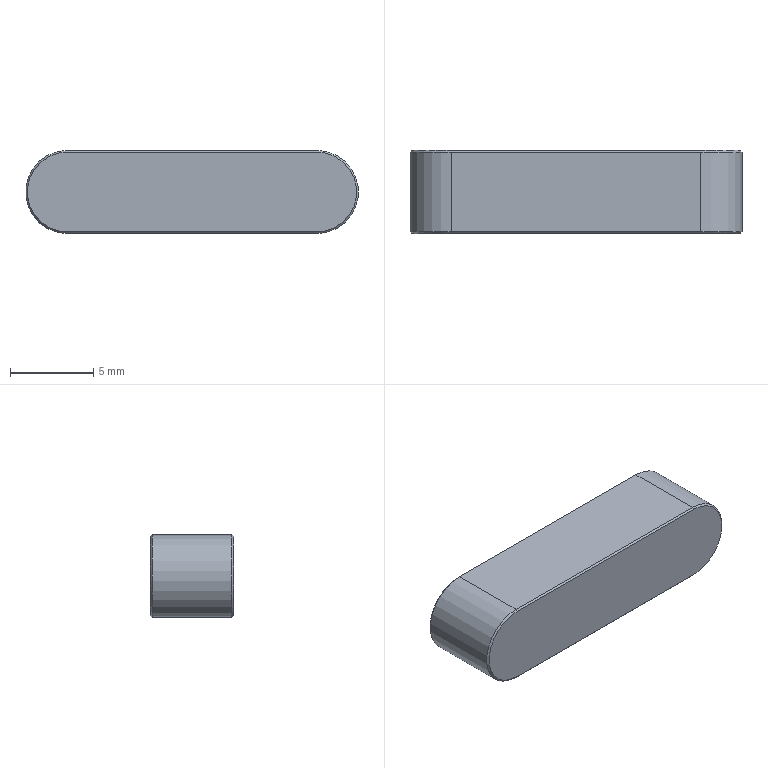Part | STEP file | Plain key (type B) 5x5x20 | 1 solid | 14 faces | box 20 x 5 x 5 mm | volume 472.72 mm3 | plane 8 | cone 4 | cylinder 2 | commonest cylinder face diameters 5 x2
STEP:
#1=CARTESIAN_POINT('',(0.,0.,0.));
#2=DIRECTION('',(0.,0.,1.));
#3=DIRECTION('',(1.,0.,0.));
#4=AXIS2_PLACEMENT_3D('',#1,#2,#3);
#5=CARTESIAN_POINT('',(-7.5,2.4,-2.5));
#6=VERTEX_POINT('',#5);
#7=CARTESIAN_POINT('',(-7.5,-2.4,-2.5));
#8=VERTEX_POINT('',#7);
#9=CARTESIAN_POINT('',(-7.5,2.5,-2.5));
#10=DIRECTION('',(0.,-1.,0.));
#11=VECTOR('',#10,1.);
#12=LINE('',#9,#11);
#13=CARTESIAN_POINT('',(-7.5,2.5,0.));
#14=DIRECTION('',(0.,-1.,0.));
#15=DIRECTION('',(0.,0.,-1.));
#16=AXIS2_PLACEMENT_3D('',#13,#14,#15);
#17=CYLINDRICAL_SURFACE('',#16,2.5);
#18=CARTESIAN_POINT('',(6.283,0.));
#19=DIRECTION('',(0.,1.));
#20=VECTOR('',#19,1.);
#21=LINE('',#18,#20);
#22=(GEOMETRIC_REPRESENTATION_CONTEXT(2)PARAMETRIC_REPRESENTATION_CONTEXT()REPRESENTATION_CONTEXT('',''));
#23=DEFINITIONAL_REPRESENTATION('',(#21),#22);
#24=PCURVE('',#17,#23);
#25=CARTESIAN_POINT('',(-7.5,2.5,-2.5));
#26=DIRECTION('',(0.,0.,1.));
#27=DIRECTION('',(1.,0.,0.));
#28=AXIS2_PLACEMENT_3D('',#25,#26,#27);
#29=PLANE('',#28);
#30=CARTESIAN_POINT('',(0.,0.));
#31=DIRECTION('',(0.,-1.));
#32=VECTOR('',#31,1.);
#33=LINE('',#30,#32);
#34=(GEOMETRIC_REPRESENTATION_CONTEXT(2)PARAMETRIC_REPRESENTATION_CONTEXT()REPRESENTATION_CONTEXT('',''));
#35=DEFINITIONAL_REPRESENTATION('',(#33),#34);
#36=PCURVE('',#29,#35);
#37=SURFACE_CURVE('',#12,(#24,#36),.PCURVE_S1.);
#38=EDGE_CURVE('',#6,#8,#37,.T.);
#39=ORIENTED_EDGE('',*,*,#38,.T.);
#40=CARTESIAN_POINT('',(-7.5,-2.4,2.5));
#41=VERTEX_POINT('',#40);
#42=CARTESIAN_POINT('',(-7.5,-2.4,0.));
#43=DIRECTION('',(0.,1.,0.));
#44=DIRECTION('',(0.,0.,1.));
#45=AXIS2_PLACEMENT_3D('',#42,#43,#44);
#46=CIRCLE('',#45,2.5);
#47=CARTESIAN_POINT('',(9.425,4.9));
#48=DIRECTION('',(-1.,0.));
#49=VECTOR('',#48,1.);
#50=LINE('',#47,#49);
#51=(GEOMETRIC_REPRESENTATION_CONTEXT(2)PARAMETRIC_REPRESENTATION_CONTEXT()REPRESENTATION_CONTEXT('',''));
#52=DEFINITIONAL_REPRESENTATION('',(#50),#51);
#53=PCURVE('',#17,#52);
#54=CARTESIAN_POINT('',(-7.5,-2.4,0.));
#55=DIRECTION('',(0.,1.,0.));
#56=DIRECTION('',(0.,0.,1.));
#57=AXIS2_PLACEMENT_3D('',#54,#55,#56);
#58=CONICAL_SURFACE('',#57,2.5,0.7854);
#59=CARTESIAN_POINT('',(0.,0.));
#60=DIRECTION('',(1.,0.));
#61=VECTOR('',#60,1.);
#62=LINE('',#59,#61);
#63=(GEOMETRIC_REPRESENTATION_CONTEXT(2)PARAMETRIC_REPRESENTATION_CONTEXT()REPRESENTATION_CONTEXT('',''));
#64=DEFINITIONAL_REPRESENTATION('',(#62),#63);
#65=PCURVE('',#58,#64);
#66=SURFACE_CURVE('',#46,(#53,#65),.PCURVE_S1.);
#67=EDGE_CURVE('',#8,#41,#66,.T.);
#68=ORIENTED_EDGE('',*,*,#67,.T.);
#69=CARTESIAN_POINT('',(-7.5,2.4,2.5));
#70=VERTEX_POINT('',#69);
#71=CARTESIAN_POINT('',(-7.5,2.5,2.5));
#72=DIRECTION('',(0.,-1.,0.));
#73=VECTOR('',#72,1.);
#74=LINE('',#71,#73);
#75=CARTESIAN_POINT('',(3.142,0.));
#76=DIRECTION('',(0.,1.));
#77=VECTOR('',#76,1.);
#78=LINE('',#75,#77);
#79=(GEOMETRIC_REPRESENTATION_CONTEXT(2)PARAMETRIC_REPRESENTATION_CONTEXT()REPRESENTATION_CONTEXT('',''));
#80=DEFINITIONAL_REPRESENTATION('',(#78),#79);
#81=PCURVE('',#17,#80);
#82=CARTESIAN_POINT('',(-7.5,2.5,2.5));
#83=DIRECTION('',(0.,0.,-1.));
#84=DIRECTION('',(-1.,0.,0.));
#85=AXIS2_PLACEMENT_3D('',#82,#83,#84);
#86=PLANE('',#85);
#87=CARTESIAN_POINT('',(0.,0.));
#88=DIRECTION('',(0.,-1.));
#89=VECTOR('',#88,1.);
#90=LINE('',#87,#89);
#91=(GEOMETRIC_REPRESENTATION_CONTEXT(2)PARAMETRIC_REPRESENTATION_CONTEXT()REPRESENTATION_CONTEXT('',''));
#92=DEFINITIONAL_REPRESENTATION('',(#90),#91);
#93=PCURVE('',#86,#92);
#94=SURFACE_CURVE('',#74,(#81,#93),.PCURVE_S1.);
#95=EDGE_CURVE('',#70,#41,#94,.T.);
#96=ORIENTED_EDGE('',*,*,#95,.F.);
#97=CARTESIAN_POINT('',(-7.5,2.4,0.));
#98=DIRECTION('',(0.,-1.,0.));
#99=DIRECTION('',(0.,0.,1.));
#100=AXIS2_PLACEMENT_3D('',#97,#98,#99);
#101=CIRCLE('',#100,2.5);
#102=CARTESIAN_POINT('',(3.142,0.1));
#103=DIRECTION('',(1.,0.));
#104=VECTOR('',#103,1.);
#105=LINE('',#102,#104);
#106=(GEOMETRIC_REPRESENTATION_CONTEXT(2)PARAMETRIC_REPRESENTATION_CONTEXT()REPRESENTATION_CONTEXT('',''));
#107=DEFINITIONAL_REPRESENTATION('',(#105),#106);
#108=PCURVE('',#17,#107);
#109=CARTESIAN_POINT('',(-7.5,2.5,0.));
#110=DIRECTION('',(0.,-1.,0.));
#111=DIRECTION('',(0.,0.,-1.));
#112=AXIS2_PLACEMENT_3D('',#109,#110,#111);
#113=CONICAL_SURFACE('',#112,2.4,0.7854);
#114=CARTESIAN_POINT('',(3.142,0.1));
#115=DIRECTION('',(1.,0.));
#116=VECTOR('',#115,1.);
#117=LINE('',#114,#116);
#118=(GEOMETRIC_REPRESENTATION_CONTEXT(2)PARAMETRIC_REPRESENTATION_CONTEXT()REPRESENTATION_CONTEXT('',''));
#119=DEFINITIONAL_REPRESENTATION('',(#117),#118);
#120=PCURVE('',#113,#119);
#121=SURFACE_CURVE('',#101,(#108,#120),.PCURVE_S1.);
#122=EDGE_CURVE('',#70,#6,#121,.T.);
#123=ORIENTED_EDGE('',*,*,#122,.T.);
#124=EDGE_LOOP('',(#39,#68,#96,#123));
#125=FACE_BOUND('',#124,.T.);
#126=ADVANCED_FACE('',(#125),#17,.T.);
#127=ORIENTED_EDGE('',*,*,#95,.T.);
#128=CARTESIAN_POINT('',(7.5,-2.4,2.5));
#129=VERTEX_POINT('',#128);
#130=CARTESIAN_POINT('',(-7.5,-2.4,2.5));
#131=DIRECTION('',(1.,0.,0.));
#132=VECTOR('',#131,1.);
#133=LINE('',#130,#132);
#134=CARTESIAN_POINT('',(0.,-4.9));
#135=DIRECTION('',(-1.,0.));
#136=VECTOR('',#135,1.);
#137=LINE('',#134,#136);
#138=(GEOMETRIC_REPRESENTATION_CONTEXT(2)PARAMETRIC_REPRESENTATION_CONTEXT()REPRESENTATION_CONTEXT('',''));
#139=DEFINITIONAL_REPRESENTATION('',(#137),#138);
#140=PCURVE('',#86,#139);
#141=CARTESIAN_POINT('',(-7.5,-2.4,2.5));
#142=DIRECTION('',(0.,0.7071,-0.7071));
#143=DIRECTION('',(1.,0.,0.));
#144=AXIS2_PLACEMENT_3D('',#141,#142,#143);
#145=PLANE('',#144);
#146=CARTESIAN_POINT('',(0.,0.));
#147=DIRECTION('',(1.,0.));
#148=VECTOR('',#147,1.);
#149=LINE('',#146,#148);
#150=(GEOMETRIC_REPRESENTATION_CONTEXT(2)PARAMETRIC_REPRESENTATION_CONTEXT()REPRESENTATION_CONTEXT('',''));
#151=DEFINITIONAL_REPRESENTATION('',(#149),#150);
#152=PCURVE('',#145,#151);
#153=SURFACE_CURVE('',#133,(#140,#152),.PCURVE_S1.);
#154=EDGE_CURVE('',#41,#129,#153,.T.);
#155=ORIENTED_EDGE('',*,*,#154,.T.);
#156=CARTESIAN_POINT('',(7.5,2.4,2.5));
#157=VERTEX_POINT('',#156);
#158=CARTESIAN_POINT('',(7.5,2.5,2.5));
#159=DIRECTION('',(0.,-1.,0.));
#160=VECTOR('',#159,1.);
#161=LINE('',#158,#160);
#162=CARTESIAN_POINT('',(-15.,0.));
#163=DIRECTION('',(0.,-1.));
#164=VECTOR('',#163,1.);
#165=LINE('',#162,#164);
#166=(GEOMETRIC_REPRESENTATION_CONTEXT(2)PARAMETRIC_REPRESENTATION_CONTEXT()REPRESENTATION_CONTEXT('',''));
#167=DEFINITIONAL_REPRESENTATION('',(#165),#166);
#168=PCURVE('',#86,#167);
#169=CARTESIAN_POINT('',(7.5,2.5,0.));
#170=DIRECTION('',(0.,-1.,0.));
#171=DIRECTION('',(0.,0.,-1.));
#172=AXIS2_PLACEMENT_3D('',#169,#170,#171);
#173=CYLINDRICAL_SURFACE('',#172,2.5);
#174=CARTESIAN_POINT('',(3.142,0.));
#175=DIRECTION('',(0.,1.));
#176=VECTOR('',#175,1.);
#177=LINE('',#174,#176);
#178=(GEOMETRIC_REPRESENTATION_CONTEXT(2)PARAMETRIC_REPRESENTATION_CONTEXT()REPRESENTATION_CONTEXT('',''));
#179=DEFINITIONAL_REPRESENTATION('',(#177),#178);
#180=PCURVE('',#173,#179);
#181=SURFACE_CURVE('',#161,(#168,#180),.PCURVE_S1.);
#182=EDGE_CURVE('',#157,#129,#181,.T.);
#183=ORIENTED_EDGE('',*,*,#182,.F.);
#184=CARTESIAN_POINT('',(-7.5,2.4,2.5));
#185=DIRECTION('',(-1.,0.,0.));
#186=VECTOR('',#185,1.);
#187=LINE('',#184,#186);
#188=CARTESIAN_POINT('',(0.,-0.1));
#189=DIRECTION('',(1.,0.));
#190=VECTOR('',#189,1.);
#191=LINE('',#188,#190);
#192=(GEOMETRIC_REPRESENTATION_CONTEXT(2)PARAMETRIC_REPRESENTATION_CONTEXT()REPRESENTATION_CONTEXT('',''));
#193=DEFINITIONAL_REPRESENTATION('',(#191),#192);
#194=PCURVE('',#86,#193);
#195=CARTESIAN_POINT('',(-7.5,2.5,2.4));
#196=DIRECTION('',(0.,0.7071,0.7071));
#197=DIRECTION('',(-1.,0.,0.));
#198=AXIS2_PLACEMENT_3D('',#195,#196,#197);
#199=PLANE('',#198);
#200=CARTESIAN_POINT('',(0.,0.1414));
#201=DIRECTION('',(1.,0.));
#202=VECTOR('',#201,1.);
#203=LINE('',#200,#202);
#204=(GEOMETRIC_REPRESENTATION_CONTEXT(2)PARAMETRIC_REPRESENTATION_CONTEXT()REPRESENTATION_CONTEXT('',''));
#205=DEFINITIONAL_REPRESENTATION('',(#203),#204);
#206=PCURVE('',#199,#205);
#207=SURFACE_CURVE('',#187,(#194,#206),.PCURVE_S1.);
#208=EDGE_CURVE('',#157,#70,#207,.T.);
#209=ORIENTED_EDGE('',*,*,#208,.T.);
#210=EDGE_LOOP('',(#127,#155,#183,#209));
#211=FACE_BOUND('',#210,.T.);
#212=ADVANCED_FACE('',(#211),#86,.F.);
#213=ORIENTED_EDGE('',*,*,#182,.T.);
#214=CARTESIAN_POINT('',(7.5,-2.4,-2.5));
#215=VERTEX_POINT('',#214);
#216=CARTESIAN_POINT('',(7.5,-2.4,0.));
#217=DIRECTION('',(0.,1.,0.));
#218=DIRECTION('',(0.,0.,1.));
#219=AXIS2_PLACEMENT_3D('',#216,#217,#218);
#220=CIRCLE('',#219,2.5);
#221=CARTESIAN_POINT('',(3.142,4.9));
#222=DIRECTION('',(-1.,0.));
#223=VECTOR('',#222,1.);
#224=LINE('',#221,#223);
#225=(GEOMETRIC_REPRESENTATION_CONTEXT(2)PARAMETRIC_REPRESENTATION_CONTEXT()REPRESENTATION_CONTEXT('',''));
#226=DEFINITIONAL_REPRESENTATION('',(#224),#225);
#227=PCURVE('',#173,#226);
#228=CARTESIAN_POINT('',(7.5,-2.4,0.));
#229=DIRECTION('',(0.,1.,0.));
#230=DIRECTION('',(0.,0.,1.));
#231=AXIS2_PLACEMENT_3D('',#228,#229,#230);
#232=CONICAL_SURFACE('',#231,2.5,0.7854);
#233=CARTESIAN_POINT('',(0.,0.));
#234=DIRECTION('',(1.,0.));
#235=VECTOR('',#234,1.);
#236=LINE('',#233,#235);
#237=(GEOMETRIC_REPRESENTATION_CONTEXT(2)PARAMETRIC_REPRESENTATION_CONTEXT()REPRESENTATION_CONTEXT('',''));
#238=DEFINITIONAL_REPRESENTATION('',(#236),#237);
#239=PCURVE('',#232,#238);
#240=SURFACE_CURVE('',#220,(#227,#239),.PCURVE_S1.);
#241=EDGE_CURVE('',#129,#215,#240,.T.);
#242=ORIENTED_EDGE('',*,*,#241,.T.);
#243=CARTESIAN_POINT('',(7.5,2.4,-2.5));
#244=VERTEX_POINT('',#243);
#245=CARTESIAN_POINT('',(7.5,2.5,-2.5));
#246=DIRECTION('',(0.,-1.,0.));
#247=VECTOR('',#246,1.);
#248=LINE('',#245,#247);
#249=CARTESIAN_POINT('',(0.,0.));
#250=DIRECTION('',(0.,1.));
#251=VECTOR('',#250,1.);
#252=LINE('',#249,#251);
#253=(GEOMETRIC_REPRESENTATION_CONTEXT(2)PARAMETRIC_REPRESENTATION_CONTEXT()REPRESENTATION_CONTEXT('',''));
#254=DEFINITIONAL_REPRESENTATION('',(#252),#253);
#255=PCURVE('',#173,#254);
#256=CARTESIAN_POINT('',(15.,0.));
#257=DIRECTION('',(0.,-1.));
#258=VECTOR('',#257,1.);
#259=LINE('',#256,#258);
#260=(GEOMETRIC_REPRESENTATION_CONTEXT(2)PARAMETRIC_REPRESENTATION_CONTEXT()REPRESENTATION_CONTEXT('',''));
#261=DEFINITIONAL_REPRESENTATION('',(#259),#260);
#262=PCURVE('',#29,#261);
#263=SURFACE_CURVE('',#248,(#255,#262),.PCURVE_S1.);
#264=EDGE_CURVE('',#244,#215,#263,.T.);
#265=ORIENTED_EDGE('',*,*,#264,.F.);
#266=CARTESIAN_POINT('',(7.5,2.4,0.));
#267=DIRECTION('',(0.,-1.,0.));
#268=DIRECTION('',(0.,0.,1.));
#269=AXIS2_PLACEMENT_3D('',#266,#267,#268);
#270=CIRCLE('',#269,2.5);
#271=CARTESIAN_POINT('',(-3.142,0.1));
#272=DIRECTION('',(1.,0.));
#273=VECTOR('',#272,1.);
#274=LINE('',#271,#273);
#275=(GEOMETRIC_REPRESENTATION_CONTEXT(2)PARAMETRIC_REPRESENTATION_CONTEXT()REPRESENTATION_CONTEXT('',''));
#276=DEFINITIONAL_REPRESENTATION('',(#274),#275);
#277=PCURVE('',#173,#276);
#278=CARTESIAN_POINT('',(7.5,2.5,0.));
#279=DIRECTION('',(0.,-1.,0.));
#280=DIRECTION('',(0.,0.,-1.));
#281=AXIS2_PLACEMENT_3D('',#278,#279,#280);
#282=CONICAL_SURFACE('',#281,2.4,0.7854);
#283=CARTESIAN_POINT('',(-3.142,0.1));
#284=DIRECTION('',(1.,0.));
#285=VECTOR('',#284,1.);
#286=LINE('',#283,#285);
#287=(GEOMETRIC_REPRESENTATION_CONTEXT(2)PARAMETRIC_REPRESENTATION_CONTEXT()REPRESENTATION_CONTEXT('',''));
#288=DEFINITIONAL_REPRESENTATION('',(#286),#287);
#289=PCURVE('',#282,#288);
#290=SURFACE_CURVE('',#270,(#277,#289),.PCURVE_S1.);
#291=EDGE_CURVE('',#244,#157,#290,.T.);
#292=ORIENTED_EDGE('',*,*,#291,.T.);
#293=EDGE_LOOP('',(#213,#242,#265,#292));
#294=FACE_BOUND('',#293,.T.);
#295=ADVANCED_FACE('',(#294),#173,.T.);
#296=ORIENTED_EDGE('',*,*,#264,.T.);
#297=CARTESIAN_POINT('',(-7.5,-2.4,-2.5));
#298=DIRECTION('',(-1.,0.,0.));
#299=VECTOR('',#298,1.);
#300=LINE('',#297,#299);
#301=CARTESIAN_POINT('',(0.,-4.9));
#302=DIRECTION('',(-1.,0.));
#303=VECTOR('',#302,1.);
#304=LINE('',#301,#303);
#305=(GEOMETRIC_REPRESENTATION_CONTEXT(2)PARAMETRIC_REPRESENTATION_CONTEXT()REPRESENTATION_CONTEXT('',''));
#306=DEFINITIONAL_REPRESENTATION('',(#304),#305);
#307=PCURVE('',#29,#306);
#308=CARTESIAN_POINT('',(-7.5,-2.4,-2.5));
#309=DIRECTION('',(0.,0.7071,0.7071));
#310=DIRECTION('',(-1.,0.,0.));
#311=AXIS2_PLACEMENT_3D('',#308,#309,#310);
#312=PLANE('',#311);
#313=CARTESIAN_POINT('',(0.,0.));
#314=DIRECTION('',(1.,0.));
#315=VECTOR('',#314,1.);
#316=LINE('',#313,#315);
#317=(GEOMETRIC_REPRESENTATION_CONTEXT(2)PARAMETRIC_REPRESENTATION_CONTEXT()REPRESENTATION_CONTEXT('',''));
#318=DEFINITIONAL_REPRESENTATION('',(#316),#317);
#319=PCURVE('',#312,#318);
#320=SURFACE_CURVE('',#300,(#307,#319),.PCURVE_S1.);
#321=EDGE_CURVE('',#215,#8,#320,.T.);
#322=ORIENTED_EDGE('',*,*,#321,.T.);
#323=ORIENTED_EDGE('',*,*,#38,.F.);
#324=CARTESIAN_POINT('',(7.5,2.4,-2.5));
#325=DIRECTION('',(1.,0.,0.));
#326=VECTOR('',#325,1.);
#327=LINE('',#324,#326);
#328=CARTESIAN_POINT('',(15.,-0.1));
#329=DIRECTION('',(1.,0.));
#330=VECTOR('',#329,1.);
#331=LINE('',#328,#330);
#332=(GEOMETRIC_REPRESENTATION_CONTEXT(2)PARAMETRIC_REPRESENTATION_CONTEXT()REPRESENTATION_CONTEXT('',''));
#333=DEFINITIONAL_REPRESENTATION('',(#331),#332);
#334=PCURVE('',#29,#333);
#335=CARTESIAN_POINT('',(-7.5,2.5,-2.4));
#336=DIRECTION('',(0.,0.7071,-0.7071));
#337=DIRECTION('',(1.,0.,0.));
#338=AXIS2_PLACEMENT_3D('',#335,#336,#337);
#339=PLANE('',#338);
#340=CARTESIAN_POINT('',(15.,0.1414));
#341=DIRECTION('',(1.,0.));
#342=VECTOR('',#341,1.);
#343=LINE('',#340,#342);
#344=(GEOMETRIC_REPRESENTATION_CONTEXT(2)PARAMETRIC_REPRESENTATION_CONTEXT()REPRESENTATION_CONTEXT('',''));
#345=DEFINITIONAL_REPRESENTATION('',(#343),#344);
#346=PCURVE('',#339,#345);
#347=SURFACE_CURVE('',#327,(#334,#346),.PCURVE_S1.);
#348=EDGE_CURVE('',#6,#244,#347,.T.);
#349=ORIENTED_EDGE('',*,*,#348,.T.);
#350=EDGE_LOOP('',(#296,#322,#323,#349));
#351=FACE_BOUND('',#350,.T.);
#352=ADVANCED_FACE('',(#351),#29,.F.);
#353=CARTESIAN_POINT('',(-7.5,2.5,-2.4));
#354=VERTEX_POINT('',#353);
#355=CARTESIAN_POINT('',(-7.5,2.5,2.4));
#356=VERTEX_POINT('',#355);
#357=CARTESIAN_POINT('',(-7.5,2.5,0.));
#358=DIRECTION('',(0.,1.,0.));
#359=DIRECTION('',(0.,0.,1.));
#360=AXIS2_PLACEMENT_3D('',#357,#358,#359);
#361=CIRCLE('',#360,2.4);
#362=CARTESIAN_POINT('',(-7.5,2.5,0.));
#363=DIRECTION('',(0.,1.,0.));
#364=DIRECTION('',(0.,0.,1.));
#365=AXIS2_PLACEMENT_3D('',#362,#363,#364);
#366=PLANE('',#365);
#367=CARTESIAN_POINT('',(0.,0.));
#368=DIRECTION('',(1.,0.));
#369=AXIS2_PLACEMENT_2D('',#367,#368);
#370=CIRCLE('',#369,2.4);
#371=(GEOMETRIC_REPRESENTATION_CONTEXT(2)PARAMETRIC_REPRESENTATION_CONTEXT()REPRESENTATION_CONTEXT('',''));
#372=DEFINITIONAL_REPRESENTATION('',(#370),#371);
#373=PCURVE('',#366,#372);
#374=CARTESIAN_POINT('',(9.425,0.));
#375=DIRECTION('',(-1.,0.));
#376=VECTOR('',#375,1.);
#377=LINE('',#374,#376);
#378=(GEOMETRIC_REPRESENTATION_CONTEXT(2)PARAMETRIC_REPRESENTATION_CONTEXT()REPRESENTATION_CONTEXT('',''));
#379=DEFINITIONAL_REPRESENTATION('',(#377),#378);
#380=PCURVE('',#113,#379);
#381=SURFACE_CURVE('',#361,(#373,#380),.PCURVE_S1.);
#382=EDGE_CURVE('',#354,#356,#381,.T.);
#383=ORIENTED_EDGE('',*,*,#382,.T.);
#384=CARTESIAN_POINT('',(7.5,2.5,2.4));
#385=VERTEX_POINT('',#384);
#386=CARTESIAN_POINT('',(7.5,2.5,2.4));
#387=DIRECTION('',(1.,0.,0.));
#388=VECTOR('',#387,1.);
#389=LINE('',#386,#388);
#390=CARTESIAN_POINT('',(2.4,15.));
#391=DIRECTION('',(0.,1.));
#392=VECTOR('',#391,1.);
#393=LINE('',#390,#392);
#394=(GEOMETRIC_REPRESENTATION_CONTEXT(2)PARAMETRIC_REPRESENTATION_CONTEXT()REPRESENTATION_CONTEXT('',''));
#395=DEFINITIONAL_REPRESENTATION('',(#393),#394);
#396=PCURVE('',#366,#395);
#397=CARTESIAN_POINT('',(-15.,0.));
#398=DIRECTION('',(-1.,0.));
#399=VECTOR('',#398,1.);
#400=LINE('',#397,#399);
#401=(GEOMETRIC_REPRESENTATION_CONTEXT(2)PARAMETRIC_REPRESENTATION_CONTEXT()REPRESENTATION_CONTEXT('',''));
#402=DEFINITIONAL_REPRESENTATION('',(#400),#401);
#403=PCURVE('',#199,#402);
#404=SURFACE_CURVE('',#389,(#396,#403),.PCURVE_S1.);
#405=EDGE_CURVE('',#356,#385,#404,.T.);
#406=ORIENTED_EDGE('',*,*,#405,.T.);
#407=CARTESIAN_POINT('',(7.5,2.5,-2.4));
#408=VERTEX_POINT('',#407);
#409=CARTESIAN_POINT('',(7.5,2.5,0.));
#410=DIRECTION('',(0.,1.,0.));
#411=DIRECTION('',(0.,0.,1.));
#412=AXIS2_PLACEMENT_3D('',#409,#410,#411);
#413=CIRCLE('',#412,2.4);
#414=CARTESIAN_POINT('',(0.,15.));
#415=DIRECTION('',(1.,0.));
#416=AXIS2_PLACEMENT_2D('',#414,#415);
#417=CIRCLE('',#416,2.4);
#418=(GEOMETRIC_REPRESENTATION_CONTEXT(2)PARAMETRIC_REPRESENTATION_CONTEXT()REPRESENTATION_CONTEXT('',''));
#419=DEFINITIONAL_REPRESENTATION('',(#417),#418);
#420=PCURVE('',#366,#419);
#421=CARTESIAN_POINT('',(3.142,0.));
#422=DIRECTION('',(-1.,0.));
#423=VECTOR('',#422,1.);
#424=LINE('',#421,#423);
#425=(GEOMETRIC_REPRESENTATION_CONTEXT(2)PARAMETRIC_REPRESENTATION_CONTEXT()REPRESENTATION_CONTEXT('',''));
#426=DEFINITIONAL_REPRESENTATION('',(#424),#425);
#427=PCURVE('',#282,#426);
#428=SURFACE_CURVE('',#413,(#420,#427),.PCURVE_S1.);
#429=EDGE_CURVE('',#385,#408,#428,.T.);
#430=ORIENTED_EDGE('',*,*,#429,.T.);
#431=CARTESIAN_POINT('',(-7.5,2.5,-2.4));
#432=DIRECTION('',(-1.,0.,0.));
#433=VECTOR('',#432,1.);
#434=LINE('',#431,#433);
#435=CARTESIAN_POINT('',(-2.4,0.));
#436=DIRECTION('',(0.,-1.));
#437=VECTOR('',#436,1.);
#438=LINE('',#435,#437);
#439=(GEOMETRIC_REPRESENTATION_CONTEXT(2)PARAMETRIC_REPRESENTATION_CONTEXT()REPRESENTATION_CONTEXT('',''));
#440=DEFINITIONAL_REPRESENTATION('',(#438),#439);
#441=PCURVE('',#366,#440);
#442=CARTESIAN_POINT('',(0.,0.));
#443=DIRECTION('',(-1.,0.));
#444=VECTOR('',#443,1.);
#445=LINE('',#442,#444);
#446=(GEOMETRIC_REPRESENTATION_CONTEXT(2)PARAMETRIC_REPRESENTATION_CONTEXT()REPRESENTATION_CONTEXT('',''));
#447=DEFINITIONAL_REPRESENTATION('',(#445),#446);
#448=PCURVE('',#339,#447);
#449=SURFACE_CURVE('',#434,(#441,#448),.PCURVE_S1.);
#450=EDGE_CURVE('',#408,#354,#449,.T.);
#451=ORIENTED_EDGE('',*,*,#450,.T.);
#452=EDGE_LOOP('',(#383,#406,#430,#451));
#453=FACE_BOUND('',#452,.T.);
#454=ADVANCED_FACE('',(#453),#366,.T.);
#455=CARTESIAN_POINT('',(7.5,-2.5,-2.4));
#456=VERTEX_POINT('',#455);
#457=CARTESIAN_POINT('',(7.5,-2.5,2.4));
#458=VERTEX_POINT('',#457);
#459=CARTESIAN_POINT('',(7.5,-2.5,0.));
#460=DIRECTION('',(0.,-1.,0.));
#461=DIRECTION('',(0.,0.,1.));
#462=AXIS2_PLACEMENT_3D('',#459,#460,#461);
#463=CIRCLE('',#462,2.4);
#464=CARTESIAN_POINT('',(-7.5,-2.5,0.));
#465=DIRECTION('',(0.,1.,0.));
#466=DIRECTION('',(0.,0.,1.));
#467=AXIS2_PLACEMENT_3D('',#464,#465,#466);
#468=PLANE('',#467);
#469=CARTESIAN_POINT('',(2.4,15.));
#470=CARTESIAN_POINT('',(2.4,10.843));
#471=CARTESIAN_POINT('',(-1.2,12.922));
#472=CARTESIAN_POINT('',(-4.8,15.));
#473=CARTESIAN_POINT('',(-1.2,17.078));
#474=CARTESIAN_POINT('',(2.4,19.157));
#475=CARTESIAN_POINT('',(2.4,15.));
#476=(BOUNDED_CURVE()B_SPLINE_CURVE(2,(#469,#470,#471,#472,#473,#474,#475),.UNSPECIFIED.,.T.,.F.)B_SPLINE_CURVE_WITH_KNOTS((1,2,2,2,2,1),(-2.094,0.,2.094,4.189,6.283,8.378),.UNSPECIFIED.)CURVE()GEOMETRIC_REPRESENTATION_ITEM()RATIONAL_B_SPLINE_CURVE((1.,0.5,1.,0.5,1.,0.5,1.))REPRESENTATION_ITEM(''));
#477=(GEOMETRIC_REPRESENTATION_CONTEXT(2)PARAMETRIC_REPRESENTATION_CONTEXT()REPRESENTATION_CONTEXT('',''));
#478=DEFINITIONAL_REPRESENTATION('',(#476),#477);
#479=PCURVE('',#468,#478);
#480=CARTESIAN_POINT('',(6.283,-0.1));
#481=DIRECTION('',(-1.,0.));
#482=VECTOR('',#481,1.);
#483=LINE('',#480,#482);
#484=(GEOMETRIC_REPRESENTATION_CONTEXT(2)PARAMETRIC_REPRESENTATION_CONTEXT()REPRESENTATION_CONTEXT('',''));
#485=DEFINITIONAL_REPRESENTATION('',(#483),#484);
#486=PCURVE('',#232,#485);
#487=SURFACE_CURVE('',#463,(#479,#486),.PCURVE_S1.);
#488=EDGE_CURVE('',#456,#458,#487,.T.);
#489=ORIENTED_EDGE('',*,*,#488,.T.);
#490=CARTESIAN_POINT('',(-7.5,-2.5,2.4));
#491=VERTEX_POINT('',#490);
#492=CARTESIAN_POINT('',(-7.5,-2.5,2.4));
#493=DIRECTION('',(-1.,0.,0.));
#494=VECTOR('',#493,1.);
#495=LINE('',#492,#494);
#496=CARTESIAN_POINT('',(2.4,0.));
#497=DIRECTION('',(0.,-1.));
#498=VECTOR('',#497,1.);
#499=LINE('',#496,#498);
#500=(GEOMETRIC_REPRESENTATION_CONTEXT(2)PARAMETRIC_REPRESENTATION_CONTEXT()REPRESENTATION_CONTEXT('',''));
#501=DEFINITIONAL_REPRESENTATION('',(#499),#500);
#502=PCURVE('',#468,#501);
#503=CARTESIAN_POINT('',(0.,0.1414));
#504=DIRECTION('',(-1.,0.));
#505=VECTOR('',#504,1.);
#506=LINE('',#503,#505);
#507=(GEOMETRIC_REPRESENTATION_CONTEXT(2)PARAMETRIC_REPRESENTATION_CONTEXT()REPRESENTATION_CONTEXT('',''));
#508=DEFINITIONAL_REPRESENTATION('',(#506),#507);
#509=PCURVE('',#145,#508);
#510=SURFACE_CURVE('',#495,(#502,#509),.PCURVE_S1.);
#511=EDGE_CURVE('',#458,#491,#510,.T.);
#512=ORIENTED_EDGE('',*,*,#511,.T.);
#513=CARTESIAN_POINT('',(-7.5,-2.5,-2.4));
#514=VERTEX_POINT('',#513);
#515=CARTESIAN_POINT('',(-7.5,-2.5,0.));
#516=DIRECTION('',(0.,-1.,0.));
#517=DIRECTION('',(0.,0.,1.));
#518=AXIS2_PLACEMENT_3D('',#515,#516,#517);
#519=CIRCLE('',#518,2.4);
#520=CARTESIAN_POINT('',(2.4,0.));
#521=CARTESIAN_POINT('',(2.4,-4.157));
#522=CARTESIAN_POINT('',(-1.2,-2.078));
#523=CARTESIAN_POINT('',(-4.8,0.));
#524=CARTESIAN_POINT('',(-1.2,2.078));
#525=CARTESIAN_POINT('',(2.4,4.157));
#526=CARTESIAN_POINT('',(2.4,0.));
#527=(BOUNDED_CURVE()B_SPLINE_CURVE(2,(#520,#521,#522,#523,#524,#525,#526),.UNSPECIFIED.,.T.,.F.)B_SPLINE_CURVE_WITH_KNOTS((1,2,2,2,2,1),(-2.094,0.,2.094,4.189,6.283,8.378),.UNSPECIFIED.)CURVE()GEOMETRIC_REPRESENTATION_ITEM()RATIONAL_B_SPLINE_CURVE((1.,0.5,1.,0.5,1.,0.5,1.))REPRESENTATION_ITEM(''));
#528=(GEOMETRIC_REPRESENTATION_CONTEXT(2)PARAMETRIC_REPRESENTATION_CONTEXT()REPRESENTATION_CONTEXT('',''));
#529=DEFINITIONAL_REPRESENTATION('',(#527),#528);
#530=PCURVE('',#468,#529);
#531=CARTESIAN_POINT('',(6.283,-0.1));
#532=DIRECTION('',(-1.,0.));
#533=VECTOR('',#532,1.);
#534=LINE('',#531,#533);
#535=(GEOMETRIC_REPRESENTATION_CONTEXT(2)PARAMETRIC_REPRESENTATION_CONTEXT()REPRESENTATION_CONTEXT('',''));
#536=DEFINITIONAL_REPRESENTATION('',(#534),#535);
#537=PCURVE('',#58,#536);
#538=SURFACE_CURVE('',#519,(#530,#537),.PCURVE_S1.);
#539=EDGE_CURVE('',#491,#514,#538,.T.);
#540=ORIENTED_EDGE('',*,*,#539,.T.);
#541=CARTESIAN_POINT('',(-7.5,-2.5,-2.4));
#542=DIRECTION('',(1.,0.,0.));
#543=VECTOR('',#542,1.);
#544=LINE('',#541,#543);
#545=CARTESIAN_POINT('',(-2.4,0.));
#546=DIRECTION('',(0.,1.));
#547=VECTOR('',#546,1.);
#548=LINE('',#545,#547);
#549=(GEOMETRIC_REPRESENTATION_CONTEXT(2)PARAMETRIC_REPRESENTATION_CONTEXT()REPRESENTATION_CONTEXT('',''));
#550=DEFINITIONAL_REPRESENTATION('',(#548),#549);
#551=PCURVE('',#468,#550);
#552=CARTESIAN_POINT('',(0.,0.1414));
#553=DIRECTION('',(-1.,0.));
#554=VECTOR('',#553,1.);
#555=LINE('',#552,#554);
#556=(GEOMETRIC_REPRESENTATION_CONTEXT(2)PARAMETRIC_REPRESENTATION_CONTEXT()REPRESENTATION_CONTEXT('',''));
#557=DEFINITIONAL_REPRESENTATION('',(#555),#556);
#558=PCURVE('',#312,#557);
#559=SURFACE_CURVE('',#544,(#551,#558),.PCURVE_S1.);
#560=EDGE_CURVE('',#514,#456,#559,.T.);
#561=ORIENTED_EDGE('',*,*,#560,.T.);
#562=EDGE_LOOP('',(#489,#512,#540,#561));
#563=FACE_BOUND('',#562,.T.);
#564=ADVANCED_FACE('',(#563),#468,.F.);
#565=CARTESIAN_POINT('',(7.5,-2.5,-2.4));
#566=DIRECTION('',(0.,0.7071,-0.7071));
#567=VECTOR('',#566,1.);
#568=LINE('',#565,#567);
#569=CARTESIAN_POINT('',(-15.,0.1414));
#570=DIRECTION('',(0.,-1.));
#571=VECTOR('',#570,1.);
#572=LINE('',#569,#571);
#573=(GEOMETRIC_REPRESENTATION_CONTEXT(2)PARAMETRIC_REPRESENTATION_CONTEXT()REPRESENTATION_CONTEXT('',''));
#574=DEFINITIONAL_REPRESENTATION('',(#572),#573);
#575=PCURVE('',#312,#574);
#576=CARTESIAN_POINT('',(3.142,-0.1));
#577=DIRECTION('',(0.,1.));
#578=VECTOR('',#577,1.);
#579=LINE('',#576,#578);
#580=(GEOMETRIC_REPRESENTATION_CONTEXT(2)PARAMETRIC_REPRESENTATION_CONTEXT()REPRESENTATION_CONTEXT('',''));
#581=DEFINITIONAL_REPRESENTATION('',(#579),#580);
#582=PCURVE('',#232,#581);
#583=SURFACE_CURVE('',#568,(#575,#582),.PCURVE_S1.);
#584=EDGE_CURVE('',#456,#215,#583,.T.);
#585=ORIENTED_EDGE('',*,*,#584,.F.);
#586=ORIENTED_EDGE('',*,*,#560,.F.);
#587=CARTESIAN_POINT('',(-7.5,-2.4,-2.5));
#588=DIRECTION('',(0.,-0.7071,0.7071));
#589=VECTOR('',#588,1.);
#590=LINE('',#587,#589);
#591=CARTESIAN_POINT('',(0.,0.));
#592=DIRECTION('',(0.,1.));
#593=VECTOR('',#592,1.);
#594=LINE('',#591,#593);
#595=(GEOMETRIC_REPRESENTATION_CONTEXT(2)PARAMETRIC_REPRESENTATION_CONTEXT()REPRESENTATION_CONTEXT('',''));
#596=DEFINITIONAL_REPRESENTATION('',(#594),#595);
#597=PCURVE('',#312,#596);
#598=CARTESIAN_POINT('',(3.142,0.));
#599=DIRECTION('',(0.,-1.));
#600=VECTOR('',#599,1.);
#601=LINE('',#598,#600);
#602=(GEOMETRIC_REPRESENTATION_CONTEXT(2)PARAMETRIC_REPRESENTATION_CONTEXT()REPRESENTATION_CONTEXT('',''));
#603=DEFINITIONAL_REPRESENTATION('',(#601),#602);
#604=PCURVE('',#58,#603);
#605=SURFACE_CURVE('',#590,(#597,#604),.PCURVE_S1.);
#606=EDGE_CURVE('',#8,#514,#605,.T.);
#607=ORIENTED_EDGE('',*,*,#606,.F.);
#608=ORIENTED_EDGE('',*,*,#321,.F.);
#609=EDGE_LOOP('',(#585,#586,#607,#608));
#610=FACE_BOUND('',#609,.T.);
#611=ADVANCED_FACE('',(#610),#312,.F.);
#612=ORIENTED_EDGE('',*,*,#606,.T.);
#613=ORIENTED_EDGE('',*,*,#539,.F.);
#614=CARTESIAN_POINT('',(-7.5,-2.4,2.5));
#615=DIRECTION('',(0.,-0.7071,-0.7071));
#616=VECTOR('',#615,1.);
#617=LINE('',#614,#616);
#618=CARTESIAN_POINT('',(6.283,0.));
#619=DIRECTION('',(0.,-1.));
#620=VECTOR('',#619,1.);
#621=LINE('',#618,#620);
#622=(GEOMETRIC_REPRESENTATION_CONTEXT(2)PARAMETRIC_REPRESENTATION_CONTEXT()REPRESENTATION_CONTEXT('',''));
#623=DEFINITIONAL_REPRESENTATION('',(#621),#622);
#624=PCURVE('',#58,#623);
#625=CARTESIAN_POINT('',(0.,0.));
#626=DIRECTION('',(0.,1.));
#627=VECTOR('',#626,1.);
#628=LINE('',#625,#627);
#629=(GEOMETRIC_REPRESENTATION_CONTEXT(2)PARAMETRIC_REPRESENTATION_CONTEXT()REPRESENTATION_CONTEXT('',''));
#630=DEFINITIONAL_REPRESENTATION('',(#628),#629);
#631=PCURVE('',#145,#630);
#632=SURFACE_CURVE('',#617,(#624,#631),.PCURVE_S1.);
#633=EDGE_CURVE('',#41,#491,#632,.T.);
#634=ORIENTED_EDGE('',*,*,#633,.F.);
#635=ORIENTED_EDGE('',*,*,#67,.F.);
#636=EDGE_LOOP('',(#612,#613,#634,#635));
#637=FACE_BOUND('',#636,.T.);
#638=ADVANCED_FACE('',(#637),#58,.T.);
#639=ORIENTED_EDGE('',*,*,#584,.T.);
#640=ORIENTED_EDGE('',*,*,#241,.F.);
#641=CARTESIAN_POINT('',(7.5,-2.5,2.4));
#642=DIRECTION('',(0.,0.7071,0.7071));
#643=VECTOR('',#642,1.);
#644=LINE('',#641,#643);
#645=CARTESIAN_POINT('',(0.,-0.1));
#646=DIRECTION('',(0.,1.));
#647=VECTOR('',#646,1.);
#648=LINE('',#645,#647);
#649=(GEOMETRIC_REPRESENTATION_CONTEXT(2)PARAMETRIC_REPRESENTATION_CONTEXT()REPRESENTATION_CONTEXT('',''));
#650=DEFINITIONAL_REPRESENTATION('',(#648),#649);
#651=PCURVE('',#232,#650);
#652=CARTESIAN_POINT('',(15.,0.1414));
#653=DIRECTION('',(0.,-1.));
#654=VECTOR('',#653,1.);
#655=LINE('',#652,#654);
#656=(GEOMETRIC_REPRESENTATION_CONTEXT(2)PARAMETRIC_REPRESENTATION_CONTEXT()REPRESENTATION_CONTEXT('',''));
#657=DEFINITIONAL_REPRESENTATION('',(#655),#656);
#658=PCURVE('',#145,#657);
#659=SURFACE_CURVE('',#644,(#651,#658),.PCURVE_S1.);
#660=EDGE_CURVE('',#458,#129,#659,.T.);
#661=ORIENTED_EDGE('',*,*,#660,.F.);
#662=ORIENTED_EDGE('',*,*,#488,.F.);
#663=EDGE_LOOP('',(#639,#640,#661,#662));
#664=FACE_BOUND('',#663,.T.);
#665=ADVANCED_FACE('',(#664),#232,.T.);
#666=ORIENTED_EDGE('',*,*,#633,.T.);
#667=ORIENTED_EDGE('',*,*,#511,.F.);
#668=ORIENTED_EDGE('',*,*,#660,.T.);
#669=ORIENTED_EDGE('',*,*,#154,.F.);
#670=EDGE_LOOP('',(#666,#667,#668,#669));
#671=FACE_BOUND('',#670,.T.);
#672=ADVANCED_FACE('',(#671),#145,.F.);
#673=CARTESIAN_POINT('',(7.5,2.4,-2.5));
#674=DIRECTION('',(0.,0.7071,0.7071));
#675=VECTOR('',#674,1.);
#676=LINE('',#673,#675);
#677=CARTESIAN_POINT('',(15.,0.1414));
#678=DIRECTION('',(0.,-1.));
#679=VECTOR('',#678,1.);
#680=LINE('',#677,#679);
#681=(GEOMETRIC_REPRESENTATION_CONTEXT(2)PARAMETRIC_REPRESENTATION_CONTEXT()REPRESENTATION_CONTEXT('',''));
#682=DEFINITIONAL_REPRESENTATION('',(#680),#681);
#683=PCURVE('',#339,#682);
#684=CARTESIAN_POINT('',(0.,0.1));
#685=DIRECTION('',(0.,-1.));
#686=VECTOR('',#685,1.);
#687=LINE('',#684,#686);
#688=(GEOMETRIC_REPRESENTATION_CONTEXT(2)PARAMETRIC_REPRESENTATION_CONTEXT()REPRESENTATION_CONTEXT('',''));
#689=DEFINITIONAL_REPRESENTATION('',(#687),#688);
#690=PCURVE('',#282,#689);
#691=SURFACE_CURVE('',#676,(#683,#690),.PCURVE_S1.);
#692=EDGE_CURVE('',#244,#408,#691,.T.);
#693=ORIENTED_EDGE('',*,*,#692,.F.);
#694=ORIENTED_EDGE('',*,*,#348,.F.);
#695=CARTESIAN_POINT('',(-7.5,2.5,-2.4));
#696=DIRECTION('',(0.,-0.7071,-0.7071));
#697=VECTOR('',#696,1.);
#698=LINE('',#695,#697);
#699=CARTESIAN_POINT('',(0.,0.));
#700=DIRECTION('',(0.,1.));
#701=VECTOR('',#700,1.);
#702=LINE('',#699,#701);
#703=(GEOMETRIC_REPRESENTATION_CONTEXT(2)PARAMETRIC_REPRESENTATION_CONTEXT()REPRESENTATION_CONTEXT('',''));
#704=DEFINITIONAL_REPRESENTATION('',(#702),#703);
#705=PCURVE('',#339,#704);
#706=CARTESIAN_POINT('',(6.283,0.));
#707=DIRECTION('',(0.,1.));
#708=VECTOR('',#707,1.);
#709=LINE('',#706,#708);
#710=(GEOMETRIC_REPRESENTATION_CONTEXT(2)PARAMETRIC_REPRESENTATION_CONTEXT()REPRESENTATION_CONTEXT('',''));
#711=DEFINITIONAL_REPRESENTATION('',(#709),#710);
#712=PCURVE('',#113,#711);
#713=SURFACE_CURVE('',#698,(#705,#712),.PCURVE_S1.);
#714=EDGE_CURVE('',#354,#6,#713,.T.);
#715=ORIENTED_EDGE('',*,*,#714,.F.);
#716=ORIENTED_EDGE('',*,*,#450,.F.);
#717=EDGE_LOOP('',(#693,#694,#715,#716));
#718=FACE_BOUND('',#717,.T.);
#719=ADVANCED_FACE('',(#718),#339,.T.);
#720=ORIENTED_EDGE('',*,*,#714,.T.);
#721=ORIENTED_EDGE('',*,*,#122,.F.);
#722=CARTESIAN_POINT('',(-7.5,2.5,2.4));
#723=DIRECTION('',(0.,-0.7071,0.7071));
#724=VECTOR('',#723,1.);
#725=LINE('',#722,#724);
#726=CARTESIAN_POINT('',(3.142,0.));
#727=DIRECTION('',(0.,1.));
#728=VECTOR('',#727,1.);
#729=LINE('',#726,#728);
#730=(GEOMETRIC_REPRESENTATION_CONTEXT(2)PARAMETRIC_REPRESENTATION_CONTEXT()REPRESENTATION_CONTEXT('',''));
#731=DEFINITIONAL_REPRESENTATION('',(#729),#730);
#732=PCURVE('',#113,#731);
#733=CARTESIAN_POINT('',(0.,0.));
#734=DIRECTION('',(0.,1.));
#735=VECTOR('',#734,1.);
#736=LINE('',#733,#735);
#737=(GEOMETRIC_REPRESENTATION_CONTEXT(2)PARAMETRIC_REPRESENTATION_CONTEXT()REPRESENTATION_CONTEXT('',''));
#738=DEFINITIONAL_REPRESENTATION('',(#736),#737);
#739=PCURVE('',#199,#738);
#740=SURFACE_CURVE('',#725,(#732,#739),.PCURVE_S1.);
#741=EDGE_CURVE('',#356,#70,#740,.T.);
#742=ORIENTED_EDGE('',*,*,#741,.F.);
#743=ORIENTED_EDGE('',*,*,#382,.F.);
#744=EDGE_LOOP('',(#720,#721,#742,#743));
#745=FACE_BOUND('',#744,.T.);
#746=ADVANCED_FACE('',(#745),#113,.T.);
#747=ORIENTED_EDGE('',*,*,#692,.T.);
#748=ORIENTED_EDGE('',*,*,#429,.F.);
#749=CARTESIAN_POINT('',(7.5,2.4,2.5));
#750=DIRECTION('',(0.,0.7071,-0.7071));
#751=VECTOR('',#750,1.);
#752=LINE('',#749,#751);
#753=CARTESIAN_POINT('',(3.142,0.1));
#754=DIRECTION('',(0.,-1.));
#755=VECTOR('',#754,1.);
#756=LINE('',#753,#755);
#757=(GEOMETRIC_REPRESENTATION_CONTEXT(2)PARAMETRIC_REPRESENTATION_CONTEXT()REPRESENTATION_CONTEXT('',''));
#758=DEFINITIONAL_REPRESENTATION('',(#756),#757);
#759=PCURVE('',#282,#758);
#760=CARTESIAN_POINT('',(-15.,0.1414));
#761=DIRECTION('',(0.,-1.));
#762=VECTOR('',#761,1.);
#763=LINE('',#760,#762);
#764=(GEOMETRIC_REPRESENTATION_CONTEXT(2)PARAMETRIC_REPRESENTATION_CONTEXT()REPRESENTATION_CONTEXT('',''));
#765=DEFINITIONAL_REPRESENTATION('',(#763),#764);
#766=PCURVE('',#199,#765);
#767=SURFACE_CURVE('',#752,(#759,#766),.PCURVE_S1.);
#768=EDGE_CURVE('',#157,#385,#767,.T.);
#769=ORIENTED_EDGE('',*,*,#768,.F.);
#770=ORIENTED_EDGE('',*,*,#291,.F.);
#771=EDGE_LOOP('',(#747,#748,#769,#770));
#772=FACE_BOUND('',#771,.T.);
#773=ADVANCED_FACE('',(#772),#282,.T.);
#774=ORIENTED_EDGE('',*,*,#741,.T.);
#775=ORIENTED_EDGE('',*,*,#208,.F.);
#776=ORIENTED_EDGE('',*,*,#768,.T.);
#777=ORIENTED_EDGE('',*,*,#405,.F.);
#778=EDGE_LOOP('',(#774,#775,#776,#777));
#779=FACE_BOUND('',#778,.T.);
#780=ADVANCED_FACE('',(#779),#199,.T.);
#781=CLOSED_SHELL('',(#126,#212,#295,#352,#454,#564,#611,#638,#665,#672,#719,#746,#773,#780));
#782=MANIFOLD_SOLID_BREP('',#781);
#783=(LENGTH_UNIT()NAMED_UNIT(*)SI_UNIT(.MILLI.,.METRE.));
#784=UNCERTAINTY_MEASURE_WITH_UNIT(LENGTH_MEASURE(0.0000001),#783,'','');
#785=(NAMED_UNIT(*)PLANE_ANGLE_UNIT()SI_UNIT($,.RADIAN.));
#786=(NAMED_UNIT(*)SI_UNIT($,.STERADIAN.)SOLID_ANGLE_UNIT());
#787=(GEOMETRIC_REPRESENTATION_CONTEXT(3)GLOBAL_UNCERTAINTY_ASSIGNED_CONTEXT((#784))GLOBAL_UNIT_ASSIGNED_CONTEXT((#783,#785,#786))REPRESENTATION_CONTEXT('',''));
#788=ADVANCED_BREP_SHAPE_REPRESENTATION('',(#4,#782),#787);